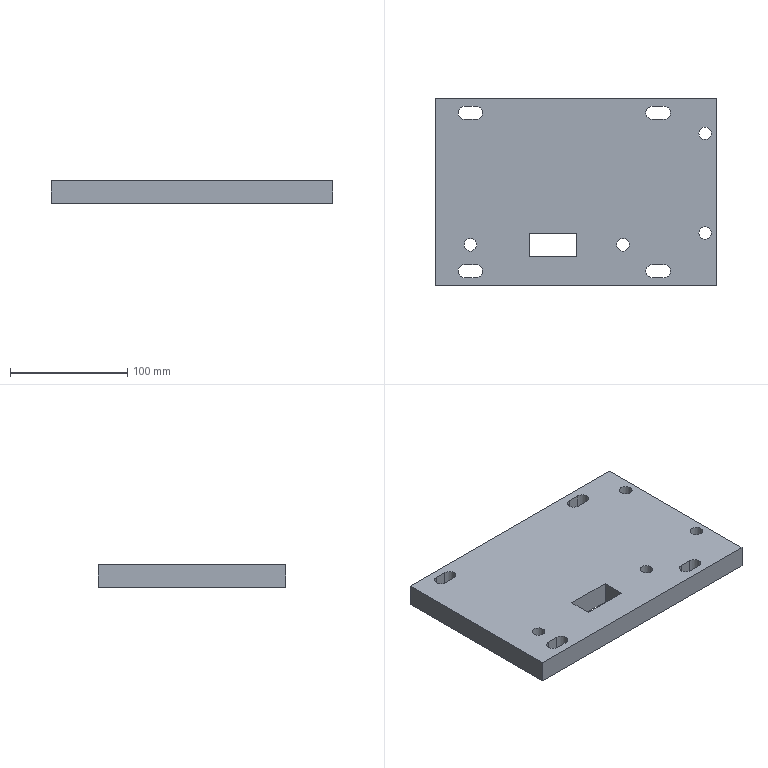Part | STEP file | YBQDJ-YB-19 | 1 solid | 38 faces | box 240 x 160 x 19 mm | volume 686478 mm3 | plane 22 | cylinder 16 | commonest cylinder face diameters 11 x8 10.7 x4 17 x4